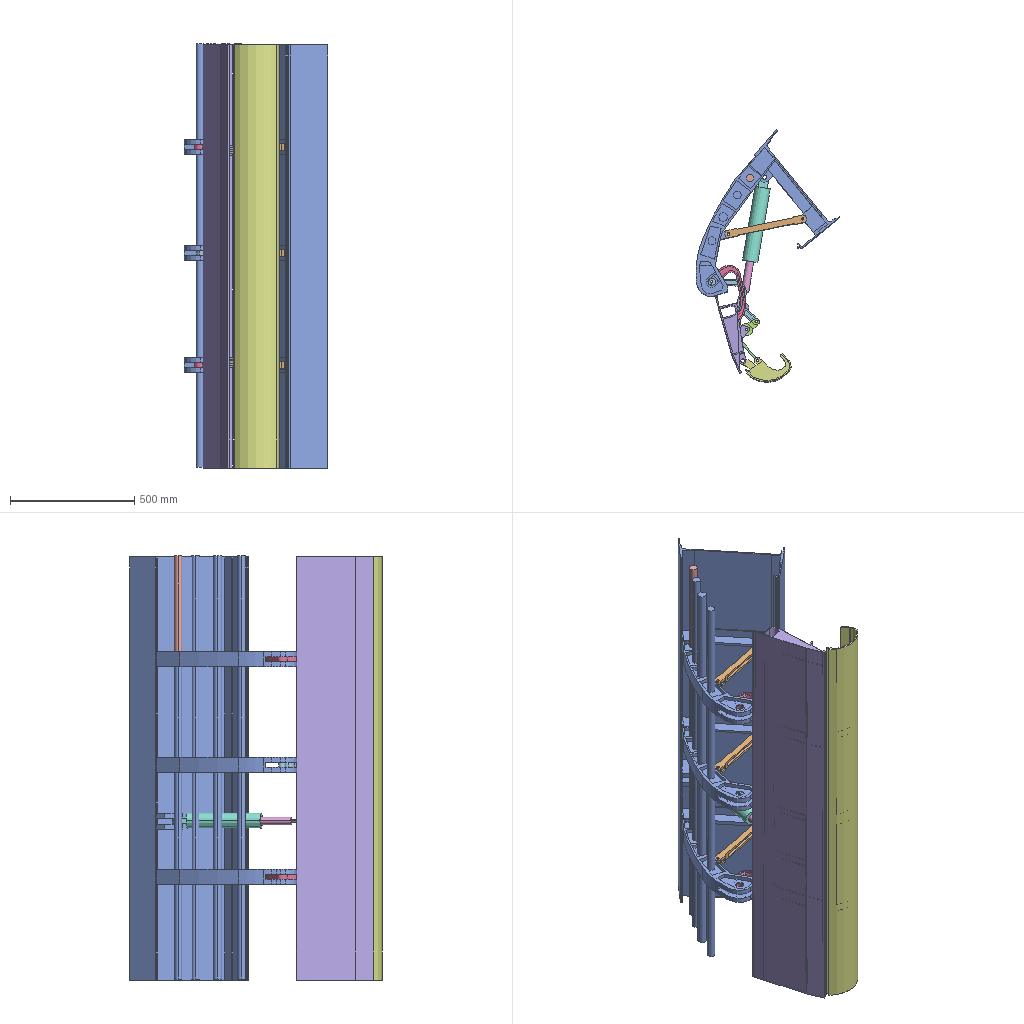Assembly | SolidWorks | 10 different items | 13 placed | box 578 x 1012 x 1705 mm
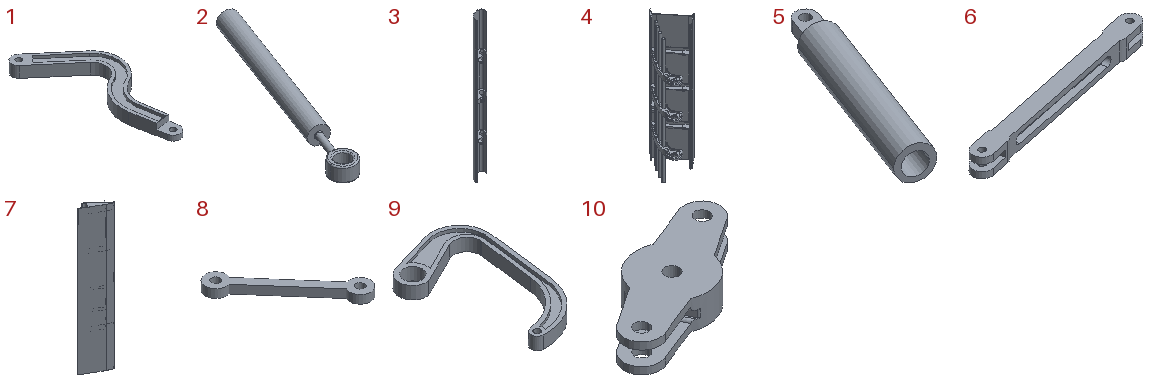Parts list (item | quantity | size | volume | features):
1 | x1 | 106.703 x 261.653 x 20 mm | 108467 mm3 | features ICE 3, Cut 1, Extrusion 1
2 | x1 | 149.428 x 332.875 x 30.111 mm | 207967 mm3 | features Fillet 2, ICE 2, Chamfer 1, Extrusion 1
3 | x1 | 168.561 x 162.568 x 1700 mm | 3528785 mm3 | features ICE 7, Extrusion 1
4 | x1 | 578.108 x 670.148 x 1705 mm | 20388998 mm3 | features ICE 25, MirrorPattern 5, Extrusion 1
5 | x1 | 167.58 x 350.157 x 61.299 mm | 596100 mm3 | features ICE 2, Extrusion 1
6 | x3 | 327.343 x 90.496 x 30 mm | 173247 mm3 | features ICE 2, Extrusion 1, MirrorPattern 1
7 | x1 | 289.155 x 223.548 x 1700 mm | 5050781 mm3 | features ICE 26, Extrusion 1
8 | x1 | 105.181 x 116.951 x 10 mm | 18015 mm3 | features Extrusion 1
9 | x2 | 141.009 x 232.349 x 20 mm | 138455 mm3 | features Extrusion 1, ICE 1
10 | x1 | 113.562 x 71.441 x 20 mm | 52250 mm3 | features ICE 3, Fillet 2, Extrusion 1
Mates (type | each side: item.copy, entity, surface, feature):
Concentric | 4.1 face cylinder Boss-Extrude23 | 6.1 face cylinder Boss-Extrude1
Coincident | 4.1 face plane Boss-Extrude23 | 6.1 face plane Cut-Extrude1
Concentric | 4.1 face cylinder Boss-Extrude24 | 6.1 face cylinder Boss-Extrude1
Concentric | 4.1 face cylinder Boss-Extrude20 | 6.2 face cylinder Boss-Extrude1
Coincident | 4.1 face plane Boss-Extrude20 | 6.2 face plane Cut-Extrude1
Concentric | 4.1 face cylinder Boss-Extrude14 | 6.3 face cylinder Boss-Extrude1
Coincident | 4.1 face plane Boss-Extrude14 | 6.3 face plane Cut-Extrude1
Concentric | 4.1 face cylinder Boss-Extrude26 | 6.3 face cylinder Boss-Extrude1
Concentric | 4.1 face cylinder Boss-Extrude25 | 6.2 face cylinder Boss-Extrude1
Concentric | 4.1 face cylinder Boss-Extrude6 | 5.1 face cylinder Boss-Extrude2
Coincident | 4.1 face plane Boss-Extrude6 | 5.1 face plane Boss-Extrude2
Concentric | 2.1 face cylinder Boss-Extrude1 | 5.1 face cylinder Cut-Extrude1
Concentric | 2.1 face cylinder Boss-Extrude4 | 7.1 face cylinder Boss-Extrude12
Coincident | 2.1 face plane Boss-Extrude4 | 7.1 face plane Boss-Extrude11
Concentric | 4.1 face cylinder Boss-Extrude2 | 9.1 face cylinder Boss-Extrude2
Coincident | 4.1 face plane Mirror6 | 9.1 face plane Boss-Extrude2
Concentric | 4.1 face cylinder Boss-Extrude3 | 9.2 face cylinder Boss-Extrude2
Coincident | 4.1 face plane Cut-Extrude4 | 9.2 face plane Boss-Extrude2
Concentric | 4.1 face cylinder Boss-Extrude4 | 1.1 face cylinder Boss-Extrude2
Parallel | 4.1 face plane Mirror5 | 1.1 face plane Boss-Extrude2
Concentric | 7.1 face cylinder Boss-Extrude33 | 9.1 face cylinder Boss-Extrude2
Concentric | 7.1 face cylinder Boss-Extrude34 | 9.2 face cylinder Boss-Extrude2
Concentric | 10.1 face cylinder Boss-Extrude3 | 8.1 face cylinder Boss-Extrude1
Coincident | 10.1 face plane Boss-Extrude3 | 8.1 face plane Boss-Extrude1
Concentric | 7.1 face cylinder Boss-Extrude6 | 3.1 face cylinder Boss-Extrude3
Coincident | 7.1 face plane Boss-Extrude5 | 3.1 face plane Boss-Extrude3
Concentric | 8.1 face cylinder Boss-Extrude1 | 3.1 face cylinder Boss-Extrude8
Coincident | 8.1 face plane Boss-Extrude1 | 3.1 face plane Boss-Extrude8
Concentric | 10.1 face cylinder Boss-Extrude1 | 7.1 face cylinder Boss-Extrude9
Coincident | 10.1 face plane Boss-Extrude1 | 7.1 face plane Boss-Extrude9
Coincident | 4.1 face plane Mirror5 | 1.1 face plane Boss-Extrude2
Concentric | 10.1 face cylinder Boss-Extrude3 | 1.1 face cylinder Boss-Extrude3
LimitDistanceDim | 5.1 face plane Boss-Extrude1 | 2.1 face plane Boss-Extrude1